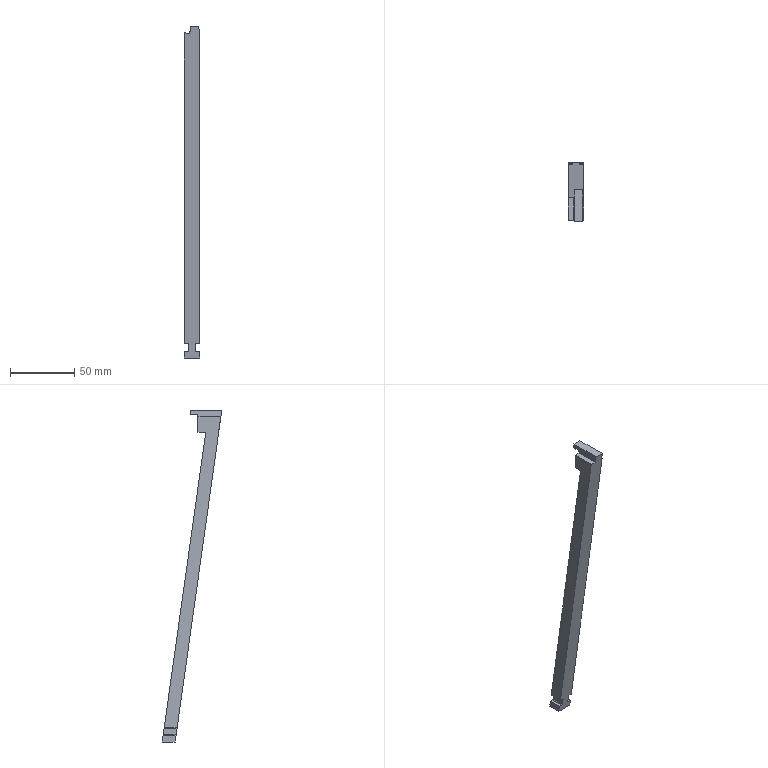Part | Creo | 1 solid | 116 faces | box 12 x 46.477 x 258.85 mm | volume 32133 mm3 | other 69 | plane 40 | cylinder 7 | commonest cylinder face diameters 1 x4 1.626 x1 2 x1 25.649 x1